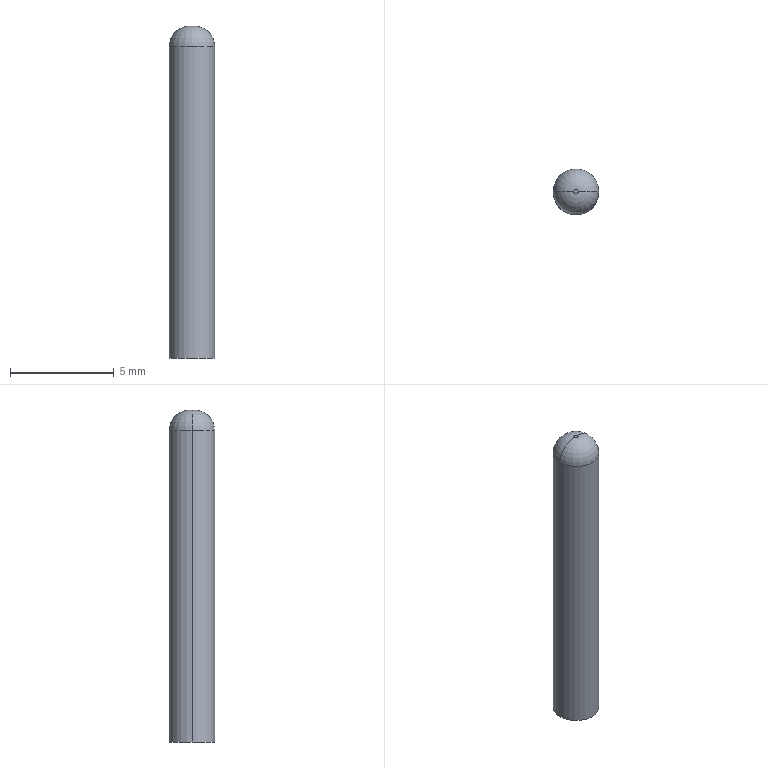Part | SolidWorks | features Attribute 3, Extrusion 1, Fillet 1 | 1 solid | 6 faces | box 2.2 x 2.2 x 16 mm | volume 59.639 mm3 | torus 2 | cylinder 2 | plane 2 | commonest cylinder face diameters 2.2 x2
STEP:
#1=CARTESIAN_POINT('',(-1.1,0.,15.));
#2=VERTEX_POINT('',#1);
#3=CARTESIAN_POINT('',(1.1,0.,15.));
#4=VERTEX_POINT('',#3);
#5=CARTESIAN_POINT('',(0.,0.,15.));
#6=DIRECTION('',(0.,0.,-1.));
#7=DIRECTION('',(1.,0.,0.));
#8=AXIS2_PLACEMENT_3D('',#5,#6,#7);
#9=CIRCLE('',#8,1.1);
#10=EDGE_CURVE('',#2,#4,#9,.T.);
#11=ORIENTED_EDGE('',*,*,#10,.F.);
#12=CARTESIAN_POINT('',(-0.1,0.,16.));
#13=VERTEX_POINT('',#12);
#14=CARTESIAN_POINT('',(-0.1,0.,15.));
#15=DIRECTION('',(0.,1.,0.));
#16=DIRECTION('',(-1.,0.,0.));
#17=AXIS2_PLACEMENT_3D('',#14,#15,#16);
#18=CIRCLE('',#17,1.);
#19=EDGE_CURVE('',#2,#13,#18,.T.);
#20=ORIENTED_EDGE('',*,*,#19,.T.);
#21=CARTESIAN_POINT('',(0.1,0.,16.));
#22=VERTEX_POINT('',#21);
#23=CARTESIAN_POINT('',(0.,0.,16.));
#24=DIRECTION('',(0.,0.,1.));
#25=DIRECTION('',(1.,0.,0.));
#26=AXIS2_PLACEMENT_3D('',#23,#24,#25);
#27=CIRCLE('',#26,0.1);
#28=EDGE_CURVE('',#22,#13,#27,.T.);
#29=ORIENTED_EDGE('',*,*,#28,.F.);
#30=CARTESIAN_POINT('',(0.1,0.,15.));
#31=DIRECTION('',(0.,-1.,0.));
#32=DIRECTION('',(0.,0.,-1.));
#33=AXIS2_PLACEMENT_3D('',#30,#31,#32);
#34=CIRCLE('',#33,1.);
#35=EDGE_CURVE('',#4,#22,#34,.T.);
#36=ORIENTED_EDGE('',*,*,#35,.F.);
#37=EDGE_LOOP('',(#11,#20,#29,#36));
#38=FACE_OUTER_BOUND('',#37,.T.);
#39=CARTESIAN_POINT('',(0.,0.,15.));
#40=DIRECTION('',(0.,0.,1.));
#41=DIRECTION('',(1.,0.,0.));
#42=AXIS2_PLACEMENT_3D('',#39,#40,#41);
#43=TOROIDAL_SURFACE('',#42,0.1,1.);
#44=ADVANCED_FACE('',(#38),#43,.T.);
#45=ORIENTED_EDGE('',*,*,#10,.T.);
#46=CARTESIAN_POINT('',(1.1,0.,0.));
#47=VERTEX_POINT('',#46);
#48=CARTESIAN_POINT('',(1.1,0.,16.));
#49=DIRECTION('',(0.,0.,-1.));
#50=VECTOR('',#49,1000.);
#51=LINE('',#48,#50);
#52=EDGE_CURVE('',#4,#47,#51,.T.);
#53=ORIENTED_EDGE('',*,*,#52,.T.);
#54=CARTESIAN_POINT('',(-1.1,0.,0.));
#55=VERTEX_POINT('',#54);
#56=CARTESIAN_POINT('',(0.,0.,0.));
#57=DIRECTION('',(0.,0.,1.));
#58=DIRECTION('',(1.,0.,0.));
#59=AXIS2_PLACEMENT_3D('',#56,#57,#58);
#60=CIRCLE('',#59,1.1);
#61=EDGE_CURVE('',#47,#55,#60,.T.);
#62=ORIENTED_EDGE('',*,*,#61,.T.);
#63=CARTESIAN_POINT('',(-1.1,0.,16.));
#64=DIRECTION('',(0.,0.,-1.));
#65=VECTOR('',#64,1000.);
#66=LINE('',#63,#65);
#67=EDGE_CURVE('',#2,#55,#66,.T.);
#68=ORIENTED_EDGE('',*,*,#67,.F.);
#69=EDGE_LOOP('',(#45,#53,#62,#68));
#70=FACE_OUTER_BOUND('',#69,.T.);
#71=CARTESIAN_POINT('',(0.,0.,16.));
#72=DIRECTION('',(0.,0.,-1.));
#73=DIRECTION('',(-1.,0.,0.));
#74=AXIS2_PLACEMENT_3D('',#71,#72,#73);
#75=CYLINDRICAL_SURFACE('',#74,1.1);
#76=ADVANCED_FACE('',(#70),#75,.T.);
#77=ORIENTED_EDGE('',*,*,#52,.F.);
#78=CARTESIAN_POINT('',(0.,0.,15.));
#79=DIRECTION('',(0.,0.,-1.));
#80=DIRECTION('',(1.,0.,0.));
#81=AXIS2_PLACEMENT_3D('',#78,#79,#80);
#82=CIRCLE('',#81,1.1);
#83=EDGE_CURVE('',#4,#2,#82,.T.);
#84=ORIENTED_EDGE('',*,*,#83,.T.);
#85=ORIENTED_EDGE('',*,*,#67,.T.);
#86=CARTESIAN_POINT('',(0.,0.,0.));
#87=DIRECTION('',(0.,0.,1.));
#88=DIRECTION('',(1.,0.,0.));
#89=AXIS2_PLACEMENT_3D('',#86,#87,#88);
#90=CIRCLE('',#89,1.1);
#91=EDGE_CURVE('',#55,#47,#90,.T.);
#92=ORIENTED_EDGE('',*,*,#91,.T.);
#93=EDGE_LOOP('',(#77,#84,#85,#92));
#94=FACE_OUTER_BOUND('',#93,.T.);
#95=CARTESIAN_POINT('',(0.,0.,16.));
#96=DIRECTION('',(0.,0.,-1.));
#97=DIRECTION('',(-1.,0.,0.));
#98=AXIS2_PLACEMENT_3D('',#95,#96,#97);
#99=CYLINDRICAL_SURFACE('',#98,1.1);
#100=ADVANCED_FACE('',(#94),#99,.T.);
#101=ORIENTED_EDGE('',*,*,#28,.T.);
#102=CARTESIAN_POINT('',(0.,0.,16.));
#103=DIRECTION('',(0.,0.,1.));
#104=DIRECTION('',(1.,0.,0.));
#105=AXIS2_PLACEMENT_3D('',#102,#103,#104);
#106=CIRCLE('',#105,0.1);
#107=EDGE_CURVE('',#13,#22,#106,.T.);
#108=ORIENTED_EDGE('',*,*,#107,.T.);
#109=EDGE_LOOP('',(#101,#108));
#110=FACE_OUTER_BOUND('',#109,.T.);
#111=CARTESIAN_POINT('',(0.,0.,16.));
#112=DIRECTION('',(0.,0.,1.));
#113=DIRECTION('',(1.,0.,0.));
#114=AXIS2_PLACEMENT_3D('',#111,#112,#113);
#115=PLANE('',#114);
#116=ADVANCED_FACE('',(#110),#115,.T.);
#117=ORIENTED_EDGE('',*,*,#91,.F.);
#118=ORIENTED_EDGE('',*,*,#61,.F.);
#119=EDGE_LOOP('',(#117,#118));
#120=FACE_OUTER_BOUND('',#119,.T.);
#121=CARTESIAN_POINT('',(0.,0.,0.));
#122=DIRECTION('',(0.,0.,1.));
#123=DIRECTION('',(1.,0.,0.));
#124=AXIS2_PLACEMENT_3D('',#121,#122,#123);
#125=PLANE('',#124);
#126=ADVANCED_FACE('',(#120),#125,.F.);
#127=ORIENTED_EDGE('',*,*,#19,.F.);
#128=ORIENTED_EDGE('',*,*,#83,.F.);
#129=ORIENTED_EDGE('',*,*,#35,.T.);
#130=ORIENTED_EDGE('',*,*,#107,.F.);
#131=EDGE_LOOP('',(#127,#128,#129,#130));
#132=FACE_OUTER_BOUND('',#131,.T.);
#133=CARTESIAN_POINT('',(0.,0.,15.));
#134=DIRECTION('',(0.,0.,1.));
#135=DIRECTION('',(1.,0.,0.));
#136=AXIS2_PLACEMENT_3D('',#133,#134,#135);
#137=TOROIDAL_SURFACE('',#136,0.1,1.);
#138=ADVANCED_FACE('',(#132),#137,.T.);
#139=CLOSED_SHELL('',(#44,#76,#100,#116,#126,#138));
#140=MANIFOLD_SOLID_BREP('',#139);
#141=CARTESIAN_POINT('',(0.,0.,0.));
#142=DIRECTION('',(0.,0.,1.));
#143=DIRECTION('',(1.,0.,0.));
#144=AXIS2_PLACEMENT_3D('',#141,#142,#143);
#145=(LENGTH_UNIT()NAMED_UNIT(*)SI_UNIT(.MILLI.,.METRE.));
#146=UNCERTAINTY_MEASURE_WITH_UNIT(LENGTH_MEASURE(0.00001),#145,'','');
#147=(NAMED_UNIT(*)PLANE_ANGLE_UNIT()SI_UNIT($,.RADIAN.));
#148=(NAMED_UNIT(*)SI_UNIT($,.STERADIAN.)SOLID_ANGLE_UNIT());
#149=(GEOMETRIC_REPRESENTATION_CONTEXT(3)GLOBAL_UNCERTAINTY_ASSIGNED_CONTEXT((#146))GLOBAL_UNIT_ASSIGNED_CONTEXT((#145,#147,#148))REPRESENTATION_CONTEXT('',''));
#150=ADVANCED_BREP_SHAPE_REPRESENTATION('',(#140,#144),#149);